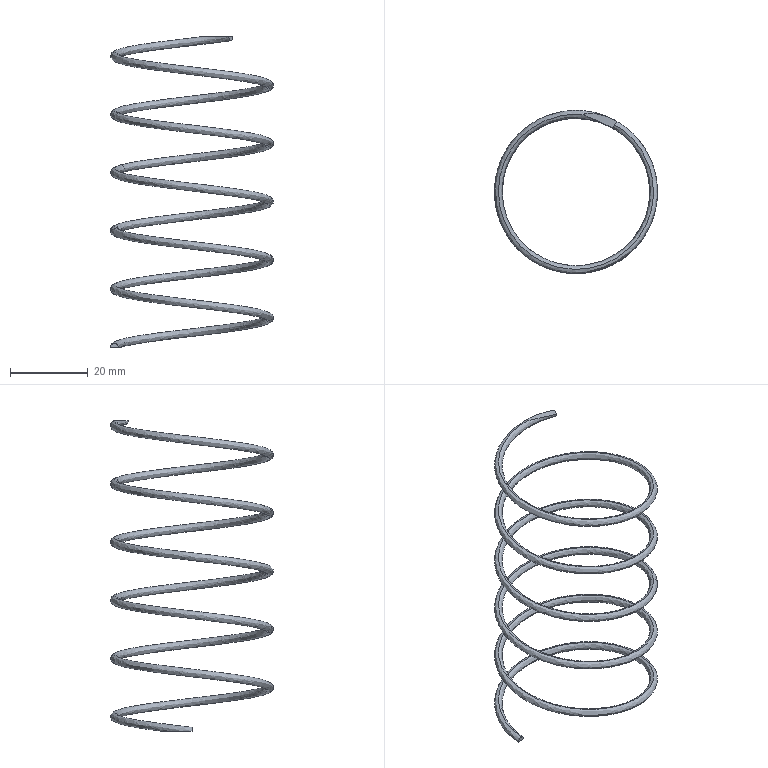Part | STEP file | 2002 Bag feed compression spring | 1 solid | 6 faces | box 42 x 42 x 80 mm | volume 2095 mm3 | plane 4 | spline 2